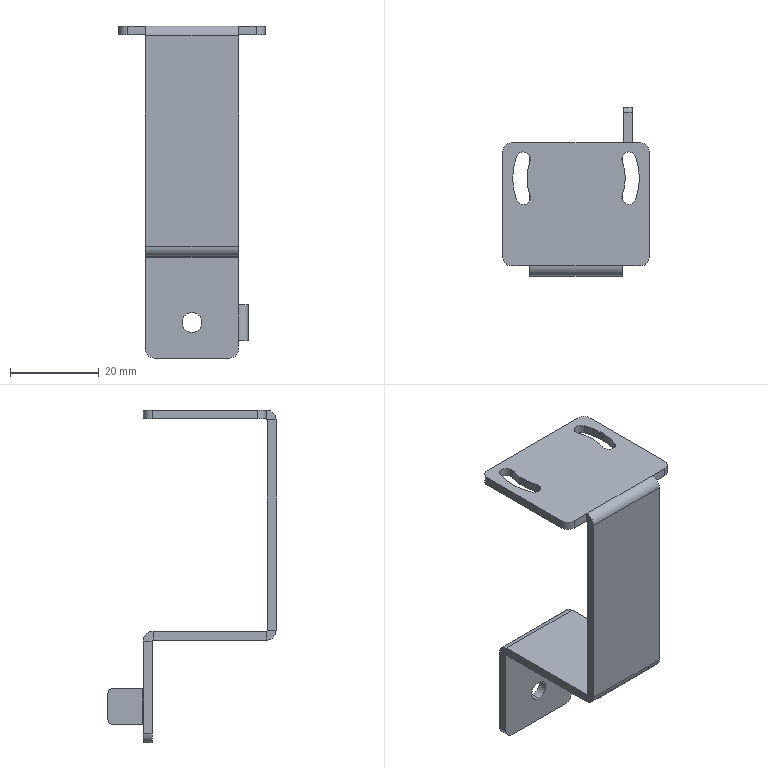Part | STEP file | Photoelectric sensor mounting plate 2 | 1 solid | 64 faces | box 33 x 38 x 75 mm | volume 6071 mm3 | plane 34 | cylinder 30 | commonest cylinder face diameters 3.2 x6 4 x6 0.4 x4 4.4 x4 22.2 x3 28.6 x3